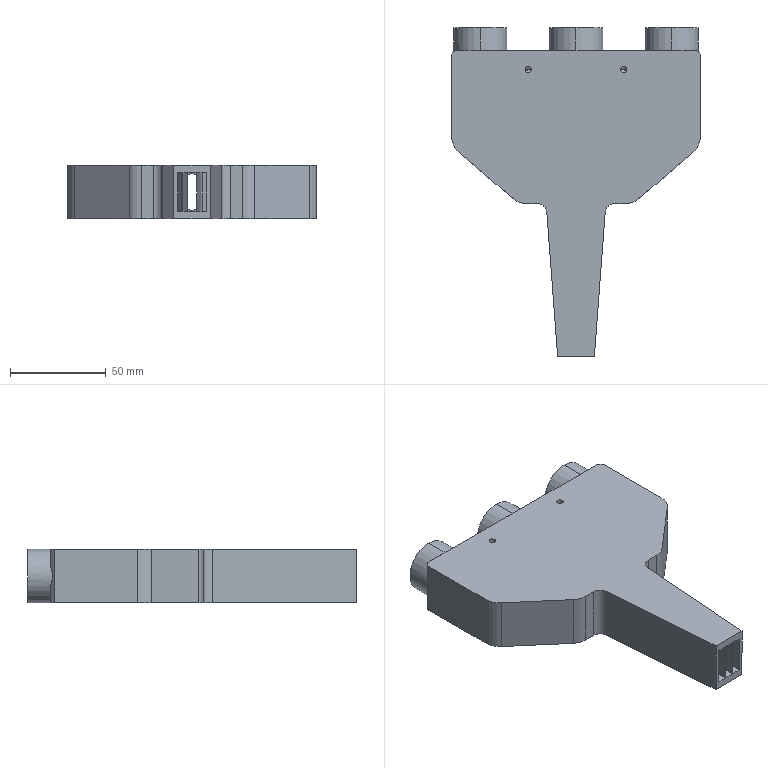Part | SolidWorks | features MirrorPattern 5, ICE 4, Cut 3, Fillet 3, SweepCut 3, 3DProfileFeature 2, HoleWzd 2, Blend 1, Chamfer 1, CombineBodies 1, Extrusion 1, LPattern 1 | 1 solid | 110 faces | box 130 x 172 x 28 mm | volume 273655 mm3 | plane 56 | cylinder 34 | cone 20 | commonest cylinder face diameters 3.3 x8 10 x6 19 x6 28 x6 20 x4 15 x2